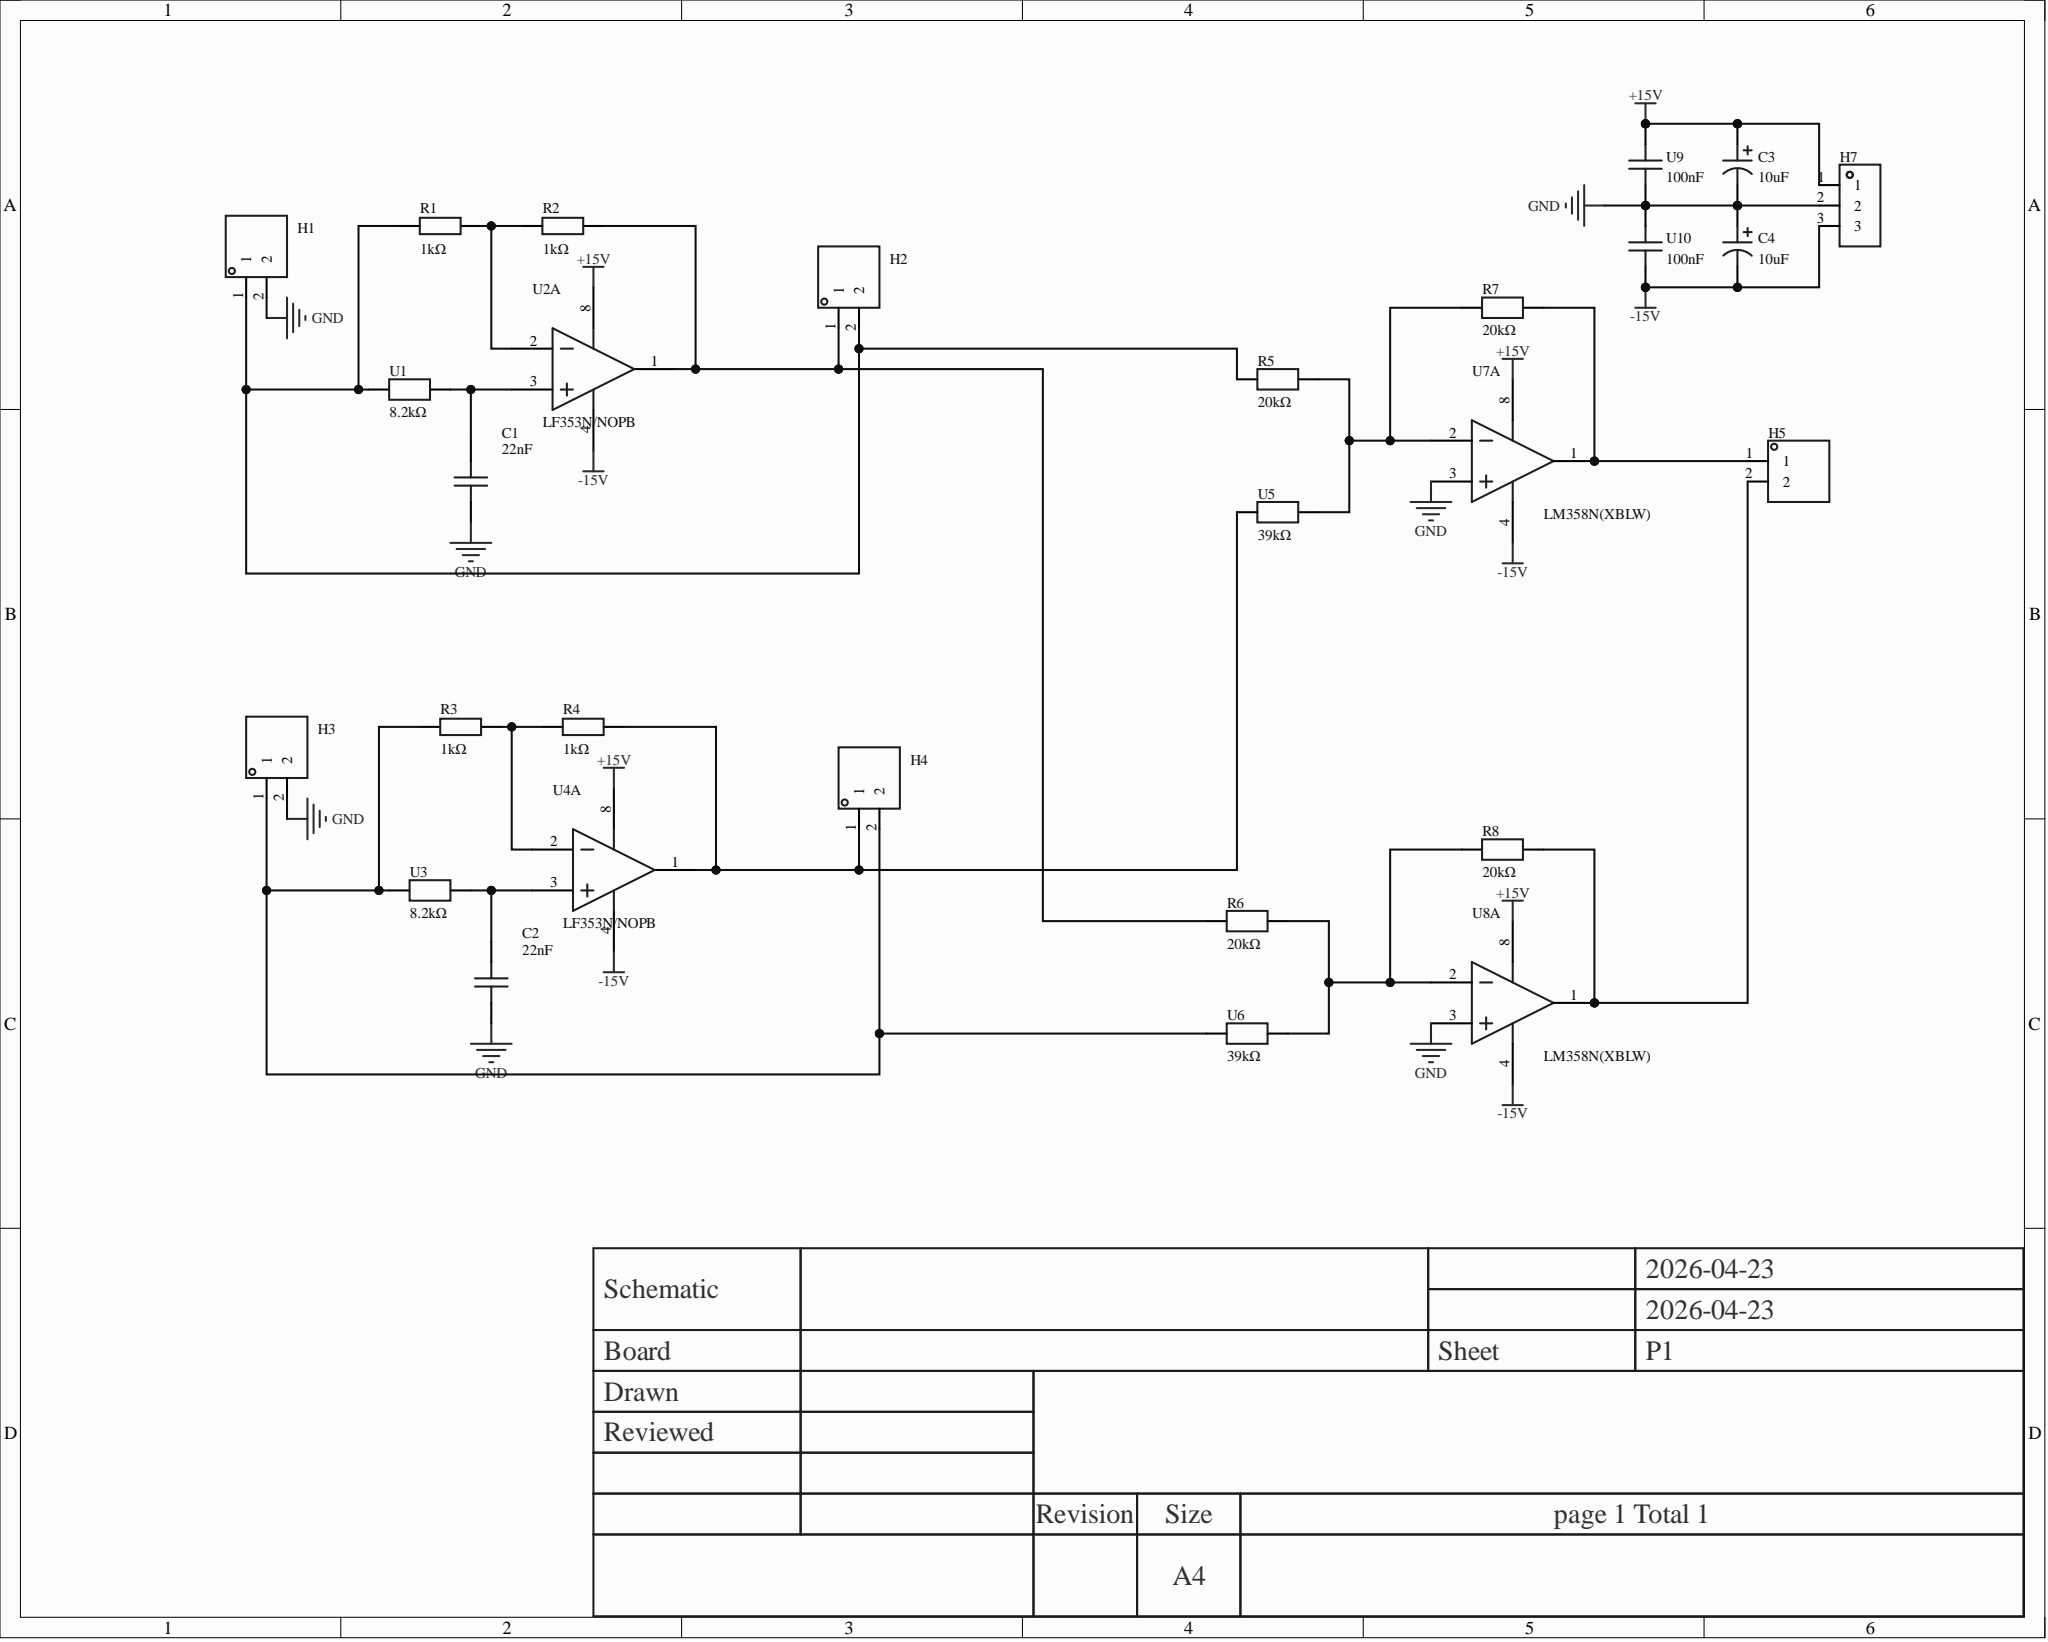Circuit board | Altium Designer | 28 parts | 15 nets
Bill of materials:
Comment,Description,Designator,Footprint,LibRef,Quantity
"22nF","","C1, C2","CAP-TH_L12.0-W4.5-P10.00-D1.0","KP223J2J1001","2"
"10uF","component 10UF50VC110GL; capacitance: 10uF; tolerance: ±20%; rated voltage: 50V; ripple current: 120mA@100KHz; equivalent series resistance (ESR): 1.6Ω;","C3, C4","CAP-TH_BD5.0-P2.00-D0.8-FD-10UF50VC110GL","10UF50VC110GL","2"
"","","H1, H2, H3, H4, H5","HDR-TH_2P-P2.54-V-M-1","HDR-M_2.54_1x2P","5"
"","","H7","HDR-TH_3P-P2.54-V-M","HDR-M_2.54_1x3P","1"
"1kΩ","component MFR0W4F1001A50; resistor type: metal film resistor; resistance: 1kΩ; tolerance: ±1%; power: 250mW; temperature coefficient: ±50ppm/?;","R1, R2, R3, R4","RES-TH_BD2.5-L6.5-P10.50-D0.6","MFR0W4F1001A50","4"
"20kΩ","","R5, R6, R7, R8","RES-TH_BD2.4-L6.3-P10.30-D0.6","RN 1/4W 20K F T/B A1","4"
"8.2kΩ","resistor type: metal film resistor; resistance: 8.2kΩ; tolerance: ±1%; power: 250mW; temperature coefficient: ±350ppm/?;","U1, U3","RES-TH_BD2.7-L6.2-P10.20-D0.4","MF1/4W-8K2±1%-ST52","2"
"LF353N/NOPB","component LF353N/NOPB; amplifier count: -; gain-bandwidth product (GBP): 4MHz; input bias current (Ib): 50pA; input offset voltage (Vos): 5mV; slew rate (SR): 13V/us; rail-to-rail: -;","U2, U4","PDIP-8_L9.6-W6.4-P2.54-LS7.6-BL","LF353N/NOPB","2"
"39kΩ","component MFR-25FRF52-39K; resistor type: metal film resistor; resistance: 39kΩ; tolerance: ±1%; power: 250mW; temperature coefficient: ±100ppm/?;","U5, U6","RES-TH_BD2.4-L6.3-P10.30-D0.6","MFR-25FRF52-39K","2"
"LM358N(XBLW)","component LM358N(XBLW); amplifier count: 2; rail-to-rail: -; gain-bandwidth product (GBW): -; input offset voltage (Vos): 5mV; slew rate (SR): 600V/ms; input bias current (Ib): 300nA;","U7, U8","PDIP-8_L9.3-W6.4-P2.54-LS7.6-BL","LM358N(XBLW)","2"
"100nF","","U9, U10","CAP-TH_L5.0-W2.5-P5.00-D1.0","100nF","2"
Netlist (Protel format):
[
C1
CAP-TH_L12.0-W4.5-P10.00-D1.0
22nF



]
[
C2
CAP-TH_L12.0-W4.5-P10.00-D1.0
22nF



]
[
C3
CAP-TH_BD5.0-P2.00-D0.8-FD-10UF50VC110GL
10uF



]
[
C4
CAP-TH_BD5.0-P2.00-D0.8-FD-10UF50VC110GL
10uF



]
[
H1
HDR-TH_2P-P2.54-V-M-1




]
[
H2
HDR-TH_2P-P2.54-V-M-1




]
[
H3
HDR-TH_2P-P2.54-V-M-1




]
[
H4
HDR-TH_2P-P2.54-V-M-1




]
[
H5
HDR-TH_2P-P2.54-V-M-1




]
[
H7
HDR-TH_3P-P2.54-V-M




]
[
R1
RES-TH_BD2.5-L6.5-P10.50-D0.6
1kΩ



]
[
R2
RES-TH_BD2.5-L6.5-P10.50-D0.6
1kΩ



]
[
R3
RES-TH_BD2.5-L6.5-P10.50-D0.6
1kΩ



]
[
R4
RES-TH_BD2.5-L6.5-P10.50-D0.6
1kΩ



]
[
R5
RES-TH_BD2.4-L6.3-P10.30-D0.6
20kΩ



]
[
R6
RES-TH_BD2.4-L6.3-P10.30-D0.6
20kΩ



]
[
R7
RES-TH_BD2.4-L6.3-P10.30-D0.6
20kΩ



]
[
R8
RES-TH_BD2.4-L6.3-P10.30-D0.6
20kΩ



]
[
U1
RES-TH_BD2.7-L6.2-P10.20-D0.4
8.2kΩ



]
[
U2
PDIP-8_L9.6-W6.4-P2.54-LS7.6-BL
LF353N/NOPB



]
[
U3
RES-TH_BD2.7-L6.2-P10.20-D0.4
8.2kΩ



]
[
U4
PDIP-8_L9.6-W6.4-P2.54-LS7.6-BL
LF353N/NOPB



]
[
U5
RES-TH_BD2.4-L6.3-P10.30-D0.6
39kΩ



]
[
U6
RES-TH_BD2.4-L6.3-P10.30-D0.6
39kΩ



]
[
U7
PDIP-8_L9.3-W6.4-P2.54-LS7.6-BL
LM358N(XBLW)



]
[
U8
PDIP-8_L9.3-W6.4-P2.54-LS7.6-BL
LM358N(XBLW)



]
[
U9
CAP-TH_L5.0-W2.5-P5.00-D1.0
100nF



]
[
U10
CAP-TH_L5.0-W2.5-P5.00-D1.0
100nF



]
(
NetR6_2
R6-2
R8-1
U6-2
U8-2
)
(
NetR5_2
R5-2
R7-1
U5-2
U7-2
)
(
NetR3_2
R3-2
R4-1
U4-2
)
(
NetR1_2
R1-2
R2-1
U2-2
)
(
NetH5_2
H5-2
R8-2
U8-1
)
(
NetH5_1
H5-1
R7-2
U7-1
)
(
NetH4_1
H4-1
R4-2
U4-1
U5-1
)
(
NetH3_1
H3-1
H4-2
R3-1
U3-1
U6-1
)
(
NetH2_1
H2-1
R2-2
R6-1
U2-1
)
(
NetH1_1
H1-1
H2-2
R1-1
R5-1
U1-1
)
(
NetC2_2
C2-2
U3-2
U4-3
)
(
NetC1_2
C1-2
U1-2
U2-3
)
(
GND
C1-1
C2-1
C3-2
C4-1
H1-2
H3-2
H7-2
U7-3
U8-3
U9-2
U10-1
)
(
-15V
C4-2
H7-3
U2-4
U4-4
U7-4
U8-4
U10-2
)
(
+15V
C3-1
H7-1
U2-8
U4-8
U7-8
U8-8
U9-1
)